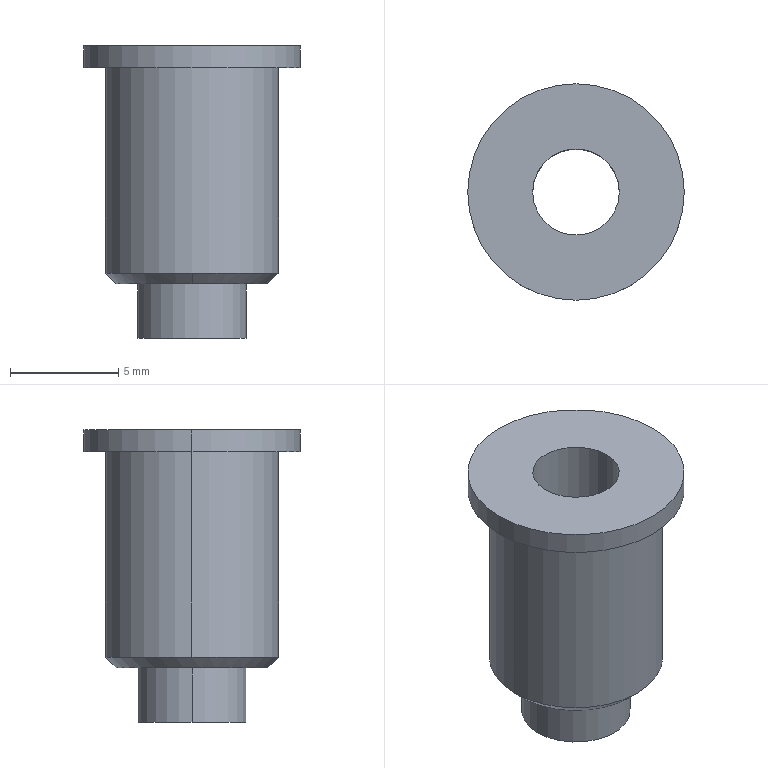Part | SolidWorks | features BaseBody 1 | 1 solid | 14 faces | box 10 x 10 x 13.5 mm | volume 457.625 mm3 | cylinder 8 | plane 4 | cone 2 | commonest cylinder face diameters 4 x2 5 x2 8 x2 10 x2
STEP:
#1=CARTESIAN_POINT('',(0.,4.,3.));
#2=VERTEX_POINT('',#1);
#3=CARTESIAN_POINT('',(-4.,0.,3.));
#4=VERTEX_POINT('',#3);
#5=CARTESIAN_POINT('',(0.,0.,3.));
#6=DIRECTION('',(0.,0.,1.));
#7=DIRECTION('',(1.,0.,0.));
#8=AXIS2_PLACEMENT_3D('',#5,#6,#7);
#9=CIRCLE('',#8,4.);
#10=EDGE_CURVE('',#2,#4,#9,.T.);
#11=ORIENTED_EDGE('',*,*,#10,.T.);
#12=CARTESIAN_POINT('',(-4.,0.,12.5));
#13=VERTEX_POINT('',#12);
#14=CARTESIAN_POINT('',(-4.,0.,2.5));
#15=DIRECTION('',(0.,0.,1.));
#16=VECTOR('',#15,1000.);
#17=LINE('',#14,#16);
#18=EDGE_CURVE('',#4,#13,#17,.T.);
#19=ORIENTED_EDGE('',*,*,#18,.T.);
#20=CARTESIAN_POINT('',(4.,0.,12.5));
#21=VERTEX_POINT('',#20);
#22=CARTESIAN_POINT('',(0.,0.,12.5));
#23=DIRECTION('',(0.,0.,-1.));
#24=DIRECTION('',(1.,0.,0.));
#25=AXIS2_PLACEMENT_3D('',#22,#23,#24);
#26=CIRCLE('',#25,4.);
#27=EDGE_CURVE('',#13,#21,#26,.T.);
#28=ORIENTED_EDGE('',*,*,#27,.T.);
#29=CARTESIAN_POINT('',(4.,0.,3.));
#30=VERTEX_POINT('',#29);
#31=CARTESIAN_POINT('',(4.,0.,2.5));
#32=DIRECTION('',(0.,0.,1.));
#33=VECTOR('',#32,1000.);
#34=LINE('',#31,#33);
#35=EDGE_CURVE('',#30,#21,#34,.T.);
#36=ORIENTED_EDGE('',*,*,#35,.F.);
#37=CARTESIAN_POINT('',(0.,0.,3.));
#38=DIRECTION('',(0.,0.,1.));
#39=DIRECTION('',(1.,0.,0.));
#40=AXIS2_PLACEMENT_3D('',#37,#38,#39);
#41=CIRCLE('',#40,4.);
#42=EDGE_CURVE('',#30,#2,#41,.T.);
#43=ORIENTED_EDGE('',*,*,#42,.T.);
#44=EDGE_LOOP('',(#11,#19,#28,#36,#43));
#45=FACE_OUTER_BOUND('',#44,.T.);
#46=CARTESIAN_POINT('',(0.,0.,2.5));
#47=DIRECTION('',(0.,0.,1.));
#48=DIRECTION('',(1.,0.,0.));
#49=AXIS2_PLACEMENT_3D('',#46,#47,#48);
#50=CYLINDRICAL_SURFACE('',#49,4.);
#51=ADVANCED_FACE('',(#45),#50,.T.);
#52=CARTESIAN_POINT('',(0.,-3.5,2.5));
#53=VERTEX_POINT('',#52);
#54=CARTESIAN_POINT('',(0.,3.5,2.5));
#55=VERTEX_POINT('',#54);
#56=CARTESIAN_POINT('',(0.,0.,2.5));
#57=DIRECTION('',(0.,0.,1.));
#58=DIRECTION('',(0.,-1.,0.));
#59=AXIS2_PLACEMENT_3D('',#56,#57,#58);
#60=CIRCLE('',#59,3.5);
#61=EDGE_CURVE('',#53,#55,#60,.T.);
#62=ORIENTED_EDGE('',*,*,#61,.T.);
#63=CARTESIAN_POINT('',(0.,4.,3.));
#64=DIRECTION('',(0.,0.7071,0.7071));
#65=VECTOR('',#64,1000.);
#66=LINE('',#63,#65);
#67=EDGE_CURVE('',#55,#2,#66,.T.);
#68=ORIENTED_EDGE('',*,*,#67,.T.);
#69=ORIENTED_EDGE('',*,*,#42,.F.);
#70=CARTESIAN_POINT('',(0.,-4.,3.));
#71=VERTEX_POINT('',#70);
#72=CARTESIAN_POINT('',(0.,0.,3.));
#73=DIRECTION('',(0.,0.,1.));
#74=DIRECTION('',(1.,0.,0.));
#75=AXIS2_PLACEMENT_3D('',#72,#73,#74);
#76=CIRCLE('',#75,4.);
#77=EDGE_CURVE('',#71,#30,#76,.T.);
#78=ORIENTED_EDGE('',*,*,#77,.F.);
#79=CARTESIAN_POINT('',(0.,-4.,3.));
#80=DIRECTION('',(0.,-0.7071,0.7071));
#81=VECTOR('',#80,1000.);
#82=LINE('',#79,#81);
#83=EDGE_CURVE('',#53,#71,#82,.T.);
#84=ORIENTED_EDGE('',*,*,#83,.F.);
#85=EDGE_LOOP('',(#62,#68,#69,#78,#84));
#86=FACE_OUTER_BOUND('',#85,.T.);
#87=CARTESIAN_POINT('',(0.,0.,3.));
#88=DIRECTION('',(0.,0.,1.));
#89=DIRECTION('',(0.,-1.,0.));
#90=AXIS2_PLACEMENT_3D('',#87,#88,#89);
#91=CONICAL_SURFACE('',#90,4.,0.7854);
#92=ADVANCED_FACE('',(#86),#91,.T.);
#93=CARTESIAN_POINT('',(-5.,0.,12.5));
#94=VERTEX_POINT('',#93);
#95=CARTESIAN_POINT('',(5.,0.,12.5));
#96=VERTEX_POINT('',#95);
#97=CARTESIAN_POINT('',(0.,0.,12.5));
#98=DIRECTION('',(0.,0.,-1.));
#99=DIRECTION('',(1.,0.,0.));
#100=AXIS2_PLACEMENT_3D('',#97,#98,#99);
#101=CIRCLE('',#100,5.);
#102=EDGE_CURVE('',#94,#96,#101,.T.);
#103=ORIENTED_EDGE('',*,*,#102,.F.);
#104=CARTESIAN_POINT('',(-5.,0.,13.5));
#105=VERTEX_POINT('',#104);
#106=CARTESIAN_POINT('',(-5.,0.,12.5));
#107=DIRECTION('',(0.,0.,1.));
#108=VECTOR('',#107,1000.);
#109=LINE('',#106,#108);
#110=EDGE_CURVE('',#94,#105,#109,.T.);
#111=ORIENTED_EDGE('',*,*,#110,.T.);
#112=CARTESIAN_POINT('',(5.,0.,13.5));
#113=VERTEX_POINT('',#112);
#114=CARTESIAN_POINT('',(0.,0.,13.5));
#115=DIRECTION('',(0.,0.,-1.));
#116=DIRECTION('',(1.,0.,0.));
#117=AXIS2_PLACEMENT_3D('',#114,#115,#116);
#118=CIRCLE('',#117,5.);
#119=EDGE_CURVE('',#105,#113,#118,.T.);
#120=ORIENTED_EDGE('',*,*,#119,.T.);
#121=CARTESIAN_POINT('',(5.,0.,12.5));
#122=DIRECTION('',(0.,0.,1.));
#123=VECTOR('',#122,1000.);
#124=LINE('',#121,#123);
#125=EDGE_CURVE('',#96,#113,#124,.T.);
#126=ORIENTED_EDGE('',*,*,#125,.F.);
#127=EDGE_LOOP('',(#103,#111,#120,#126));
#128=FACE_OUTER_BOUND('',#127,.T.);
#129=CARTESIAN_POINT('',(0.,0.,12.5));
#130=DIRECTION('',(0.,0.,1.));
#131=DIRECTION('',(1.,0.,0.));
#132=AXIS2_PLACEMENT_3D('',#129,#130,#131);
#133=CYLINDRICAL_SURFACE('',#132,5.);
#134=ADVANCED_FACE('',(#128),#133,.T.);
#135=CARTESIAN_POINT('',(2.5,0.,0.));
#136=VERTEX_POINT('',#135);
#137=CARTESIAN_POINT('',(-2.5,0.,0.));
#138=VERTEX_POINT('',#137);
#139=CARTESIAN_POINT('',(0.,0.,0.));
#140=DIRECTION('',(0.,0.,1.));
#141=DIRECTION('',(1.,0.,0.));
#142=AXIS2_PLACEMENT_3D('',#139,#140,#141);
#143=CIRCLE('',#142,2.5);
#144=EDGE_CURVE('',#136,#138,#143,.T.);
#145=ORIENTED_EDGE('',*,*,#144,.T.);
#146=CARTESIAN_POINT('',(-2.5,0.,2.5));
#147=VERTEX_POINT('',#146);
#148=CARTESIAN_POINT('',(-2.5,0.,0.));
#149=DIRECTION('',(0.,0.,1.));
#150=VECTOR('',#149,1000.);
#151=LINE('',#148,#150);
#152=EDGE_CURVE('',#138,#147,#151,.T.);
#153=ORIENTED_EDGE('',*,*,#152,.T.);
#154=CARTESIAN_POINT('',(2.5,0.,2.5));
#155=VERTEX_POINT('',#154);
#156=CARTESIAN_POINT('',(0.,0.,2.5));
#157=DIRECTION('',(0.,0.,1.));
#158=DIRECTION('',(1.,0.,0.));
#159=AXIS2_PLACEMENT_3D('',#156,#157,#158);
#160=CIRCLE('',#159,2.5);
#161=EDGE_CURVE('',#155,#147,#160,.T.);
#162=ORIENTED_EDGE('',*,*,#161,.F.);
#163=CARTESIAN_POINT('',(2.5,0.,0.));
#164=DIRECTION('',(0.,0.,1.));
#165=VECTOR('',#164,1000.);
#166=LINE('',#163,#165);
#167=EDGE_CURVE('',#136,#155,#166,.T.);
#168=ORIENTED_EDGE('',*,*,#167,.F.);
#169=EDGE_LOOP('',(#145,#153,#162,#168));
#170=FACE_OUTER_BOUND('',#169,.T.);
#171=CARTESIAN_POINT('',(0.,0.,0.));
#172=DIRECTION('',(0.,0.,1.));
#173=DIRECTION('',(1.,0.,0.));
#174=AXIS2_PLACEMENT_3D('',#171,#172,#173);
#175=CYLINDRICAL_SURFACE('',#174,2.5);
#176=ADVANCED_FACE('',(#170),#175,.T.);
#177=CARTESIAN_POINT('',(-2.,0.,0.));
#178=VERTEX_POINT('',#177);
#179=CARTESIAN_POINT('',(2.,0.,0.));
#180=VERTEX_POINT('',#179);
#181=CARTESIAN_POINT('',(0.,0.,0.));
#182=DIRECTION('',(0.,0.,1.));
#183=DIRECTION('',(1.,0.,0.));
#184=AXIS2_PLACEMENT_3D('',#181,#182,#183);
#185=CIRCLE('',#184,2.);
#186=EDGE_CURVE('',#178,#180,#185,.T.);
#187=ORIENTED_EDGE('',*,*,#186,.F.);
#188=CARTESIAN_POINT('',(-2.,0.,13.5));
#189=VERTEX_POINT('',#188);
#190=CARTESIAN_POINT('',(-2.,0.,-6.051));
#191=DIRECTION('',(0.,0.,1.));
#192=VECTOR('',#191,1000.);
#193=LINE('',#190,#192);
#194=EDGE_CURVE('',#178,#189,#193,.T.);
#195=ORIENTED_EDGE('',*,*,#194,.T.);
#196=CARTESIAN_POINT('',(2.,0.,13.5));
#197=VERTEX_POINT('',#196);
#198=CARTESIAN_POINT('',(0.,0.,13.5));
#199=DIRECTION('',(0.,0.,1.));
#200=DIRECTION('',(1.,0.,0.));
#201=AXIS2_PLACEMENT_3D('',#198,#199,#200);
#202=CIRCLE('',#201,2.);
#203=EDGE_CURVE('',#189,#197,#202,.T.);
#204=ORIENTED_EDGE('',*,*,#203,.T.);
#205=CARTESIAN_POINT('',(2.,0.,-6.051));
#206=DIRECTION('',(0.,0.,1.));
#207=VECTOR('',#206,1000.);
#208=LINE('',#205,#207);
#209=EDGE_CURVE('',#180,#197,#208,.T.);
#210=ORIENTED_EDGE('',*,*,#209,.F.);
#211=EDGE_LOOP('',(#187,#195,#204,#210));
#212=FACE_OUTER_BOUND('',#211,.T.);
#213=CARTESIAN_POINT('',(0.,0.,-6.051));
#214=DIRECTION('',(0.,0.,1.));
#215=DIRECTION('',(1.,0.,0.));
#216=AXIS2_PLACEMENT_3D('',#213,#214,#215);
#217=CYLINDRICAL_SURFACE('',#216,2.);
#218=ADVANCED_FACE('',(#212),#217,.F.);
#219=ORIENTED_EDGE('',*,*,#18,.F.);
#220=CARTESIAN_POINT('',(0.,0.,3.));
#221=DIRECTION('',(0.,0.,1.));
#222=DIRECTION('',(1.,0.,0.));
#223=AXIS2_PLACEMENT_3D('',#220,#221,#222);
#224=CIRCLE('',#223,4.);
#225=EDGE_CURVE('',#4,#71,#224,.T.);
#226=ORIENTED_EDGE('',*,*,#225,.T.);
#227=ORIENTED_EDGE('',*,*,#77,.T.);
#228=ORIENTED_EDGE('',*,*,#35,.T.);
#229=CARTESIAN_POINT('',(0.,0.,12.5));
#230=DIRECTION('',(0.,0.,-1.));
#231=DIRECTION('',(1.,0.,0.));
#232=AXIS2_PLACEMENT_3D('',#229,#230,#231);
#233=CIRCLE('',#232,4.);
#234=EDGE_CURVE('',#21,#13,#233,.T.);
#235=ORIENTED_EDGE('',*,*,#234,.T.);
#236=EDGE_LOOP('',(#219,#226,#227,#228,#235));
#237=FACE_OUTER_BOUND('',#236,.T.);
#238=CARTESIAN_POINT('',(0.,0.,2.5));
#239=DIRECTION('',(0.,0.,1.));
#240=DIRECTION('',(1.,0.,0.));
#241=AXIS2_PLACEMENT_3D('',#238,#239,#240);
#242=CYLINDRICAL_SURFACE('',#241,4.);
#243=ADVANCED_FACE('',(#237),#242,.T.);
#244=ORIENTED_EDGE('',*,*,#67,.F.);
#245=CARTESIAN_POINT('',(0.,0.,2.5));
#246=DIRECTION('',(0.,0.,1.));
#247=DIRECTION('',(0.,-1.,0.));
#248=AXIS2_PLACEMENT_3D('',#245,#246,#247);
#249=CIRCLE('',#248,3.5);
#250=EDGE_CURVE('',#55,#53,#249,.T.);
#251=ORIENTED_EDGE('',*,*,#250,.T.);
#252=ORIENTED_EDGE('',*,*,#83,.T.);
#253=ORIENTED_EDGE('',*,*,#225,.F.);
#254=ORIENTED_EDGE('',*,*,#10,.F.);
#255=EDGE_LOOP('',(#244,#251,#252,#253,#254));
#256=FACE_OUTER_BOUND('',#255,.T.);
#257=CARTESIAN_POINT('',(0.,0.,3.));
#258=DIRECTION('',(0.,0.,1.));
#259=DIRECTION('',(0.,-1.,0.));
#260=AXIS2_PLACEMENT_3D('',#257,#258,#259);
#261=CONICAL_SURFACE('',#260,4.,0.7854);
#262=ADVANCED_FACE('',(#256),#261,.T.);
#263=ORIENTED_EDGE('',*,*,#234,.F.);
#264=ORIENTED_EDGE('',*,*,#27,.F.);
#265=EDGE_LOOP('',(#263,#264));
#266=FACE_BOUND('',#265,.T.);
#267=CARTESIAN_POINT('',(0.,0.,12.5));
#268=DIRECTION('',(0.,0.,-1.));
#269=DIRECTION('',(1.,0.,0.));
#270=AXIS2_PLACEMENT_3D('',#267,#268,#269);
#271=CIRCLE('',#270,5.);
#272=EDGE_CURVE('',#96,#94,#271,.T.);
#273=ORIENTED_EDGE('',*,*,#272,.T.);
#274=ORIENTED_EDGE('',*,*,#102,.T.);
#275=EDGE_LOOP('',(#273,#274));
#276=FACE_OUTER_BOUND('',#275,.T.);
#277=CARTESIAN_POINT('',(0.,0.,12.5));
#278=DIRECTION('',(0.,0.,-1.));
#279=DIRECTION('',(-1.,0.,0.));
#280=AXIS2_PLACEMENT_3D('',#277,#278,#279);
#281=PLANE('',#280);
#282=ADVANCED_FACE('',(#266,#276),#281,.T.);
#283=ORIENTED_EDGE('',*,*,#161,.T.);
#284=CARTESIAN_POINT('',(0.,0.,2.5));
#285=DIRECTION('',(0.,0.,1.));
#286=DIRECTION('',(1.,0.,0.));
#287=AXIS2_PLACEMENT_3D('',#284,#285,#286);
#288=CIRCLE('',#287,2.5);
#289=EDGE_CURVE('',#147,#155,#288,.T.);
#290=ORIENTED_EDGE('',*,*,#289,.T.);
#291=EDGE_LOOP('',(#283,#290));
#292=FACE_BOUND('',#291,.T.);
#293=ORIENTED_EDGE('',*,*,#61,.F.);
#294=ORIENTED_EDGE('',*,*,#250,.F.);
#295=EDGE_LOOP('',(#293,#294));
#296=FACE_OUTER_BOUND('',#295,.T.);
#297=CARTESIAN_POINT('',(0.,0.,2.5));
#298=DIRECTION('',(0.,0.,-1.));
#299=DIRECTION('',(-1.,0.,0.));
#300=AXIS2_PLACEMENT_3D('',#297,#298,#299);
#301=PLANE('',#300);
#302=ADVANCED_FACE('',(#292,#296),#301,.T.);
#303=ORIENTED_EDGE('',*,*,#110,.F.);
#304=ORIENTED_EDGE('',*,*,#272,.F.);
#305=ORIENTED_EDGE('',*,*,#125,.T.);
#306=CARTESIAN_POINT('',(0.,0.,13.5));
#307=DIRECTION('',(0.,0.,-1.));
#308=DIRECTION('',(1.,0.,0.));
#309=AXIS2_PLACEMENT_3D('',#306,#307,#308);
#310=CIRCLE('',#309,5.);
#311=EDGE_CURVE('',#113,#105,#310,.T.);
#312=ORIENTED_EDGE('',*,*,#311,.T.);
#313=EDGE_LOOP('',(#303,#304,#305,#312));
#314=FACE_OUTER_BOUND('',#313,.T.);
#315=CARTESIAN_POINT('',(0.,0.,12.5));
#316=DIRECTION('',(0.,0.,1.));
#317=DIRECTION('',(1.,0.,0.));
#318=AXIS2_PLACEMENT_3D('',#315,#316,#317);
#319=CYLINDRICAL_SURFACE('',#318,5.);
#320=ADVANCED_FACE('',(#314),#319,.T.);
#321=ORIENTED_EDGE('',*,*,#152,.F.);
#322=CARTESIAN_POINT('',(0.,0.,0.));
#323=DIRECTION('',(0.,0.,1.));
#324=DIRECTION('',(1.,0.,0.));
#325=AXIS2_PLACEMENT_3D('',#322,#323,#324);
#326=CIRCLE('',#325,2.5);
#327=EDGE_CURVE('',#138,#136,#326,.T.);
#328=ORIENTED_EDGE('',*,*,#327,.T.);
#329=ORIENTED_EDGE('',*,*,#167,.T.);
#330=ORIENTED_EDGE('',*,*,#289,.F.);
#331=EDGE_LOOP('',(#321,#328,#329,#330));
#332=FACE_OUTER_BOUND('',#331,.T.);
#333=CARTESIAN_POINT('',(0.,0.,0.));
#334=DIRECTION('',(0.,0.,1.));
#335=DIRECTION('',(1.,0.,0.));
#336=AXIS2_PLACEMENT_3D('',#333,#334,#335);
#337=CYLINDRICAL_SURFACE('',#336,2.5);
#338=ADVANCED_FACE('',(#332),#337,.T.);
#339=CARTESIAN_POINT('',(0.,0.,13.5));
#340=DIRECTION('',(0.,0.,1.));
#341=DIRECTION('',(1.,0.,0.));
#342=AXIS2_PLACEMENT_3D('',#339,#340,#341);
#343=CIRCLE('',#342,2.);
#344=EDGE_CURVE('',#197,#189,#343,.T.);
#345=ORIENTED_EDGE('',*,*,#344,.F.);
#346=ORIENTED_EDGE('',*,*,#203,.F.);
#347=EDGE_LOOP('',(#345,#346));
#348=FACE_BOUND('',#347,.T.);
#349=ORIENTED_EDGE('',*,*,#311,.F.);
#350=ORIENTED_EDGE('',*,*,#119,.F.);
#351=EDGE_LOOP('',(#349,#350));
#352=FACE_OUTER_BOUND('',#351,.T.);
#353=CARTESIAN_POINT('',(0.,0.,13.5));
#354=DIRECTION('',(0.,0.,-1.));
#355=DIRECTION('',(-1.,0.,0.));
#356=AXIS2_PLACEMENT_3D('',#353,#354,#355);
#357=PLANE('',#356);
#358=ADVANCED_FACE('',(#348,#352),#357,.F.);
#359=CARTESIAN_POINT('',(0.,0.,0.));
#360=DIRECTION('',(0.,0.,1.));
#361=DIRECTION('',(1.,0.,0.));
#362=AXIS2_PLACEMENT_3D('',#359,#360,#361);
#363=CIRCLE('',#362,2.);
#364=EDGE_CURVE('',#180,#178,#363,.T.);
#365=ORIENTED_EDGE('',*,*,#364,.T.);
#366=ORIENTED_EDGE('',*,*,#186,.T.);
#367=EDGE_LOOP('',(#365,#366));
#368=FACE_BOUND('',#367,.T.);
#369=ORIENTED_EDGE('',*,*,#144,.F.);
#370=ORIENTED_EDGE('',*,*,#327,.F.);
#371=EDGE_LOOP('',(#369,#370));
#372=FACE_OUTER_BOUND('',#371,.T.);
#373=CARTESIAN_POINT('',(0.,0.,0.));
#374=DIRECTION('',(0.,0.,-1.));
#375=DIRECTION('',(-1.,0.,0.));
#376=AXIS2_PLACEMENT_3D('',#373,#374,#375);
#377=PLANE('',#376);
#378=ADVANCED_FACE('',(#368,#372),#377,.T.);
#379=ORIENTED_EDGE('',*,*,#194,.F.);
#380=ORIENTED_EDGE('',*,*,#364,.F.);
#381=ORIENTED_EDGE('',*,*,#209,.T.);
#382=ORIENTED_EDGE('',*,*,#344,.T.);
#383=EDGE_LOOP('',(#379,#380,#381,#382));
#384=FACE_OUTER_BOUND('',#383,.T.);
#385=CARTESIAN_POINT('',(0.,0.,-6.051));
#386=DIRECTION('',(0.,0.,1.));
#387=DIRECTION('',(1.,0.,0.));
#388=AXIS2_PLACEMENT_3D('',#385,#386,#387);
#389=CYLINDRICAL_SURFACE('',#388,2.);
#390=ADVANCED_FACE('',(#384),#389,.F.);
#391=CLOSED_SHELL('',(#51,#92,#134,#176,#218,#243,#262,#282,#302,#320,#338,#358,#378,#390));
#392=MANIFOLD_SOLID_BREP('',#391);
#393=CARTESIAN_POINT('',(0.,0.,0.));
#394=DIRECTION('',(0.,0.,1.));
#395=DIRECTION('',(1.,0.,0.));
#396=AXIS2_PLACEMENT_3D('',#393,#394,#395);
#397=(LENGTH_UNIT()NAMED_UNIT(*)SI_UNIT(.MILLI.,.METRE.));
#398=UNCERTAINTY_MEASURE_WITH_UNIT(LENGTH_MEASURE(0.00001),#397,'','');
#399=(NAMED_UNIT(*)PLANE_ANGLE_UNIT()SI_UNIT($,.RADIAN.));
#400=(NAMED_UNIT(*)SI_UNIT($,.STERADIAN.)SOLID_ANGLE_UNIT());
#401=(GEOMETRIC_REPRESENTATION_CONTEXT(3)GLOBAL_UNCERTAINTY_ASSIGNED_CONTEXT((#398))GLOBAL_UNIT_ASSIGNED_CONTEXT((#397,#399,#400))REPRESENTATION_CONTEXT('',''));
#402=ADVANCED_BREP_SHAPE_REPRESENTATION('',(#392,#396),#401);